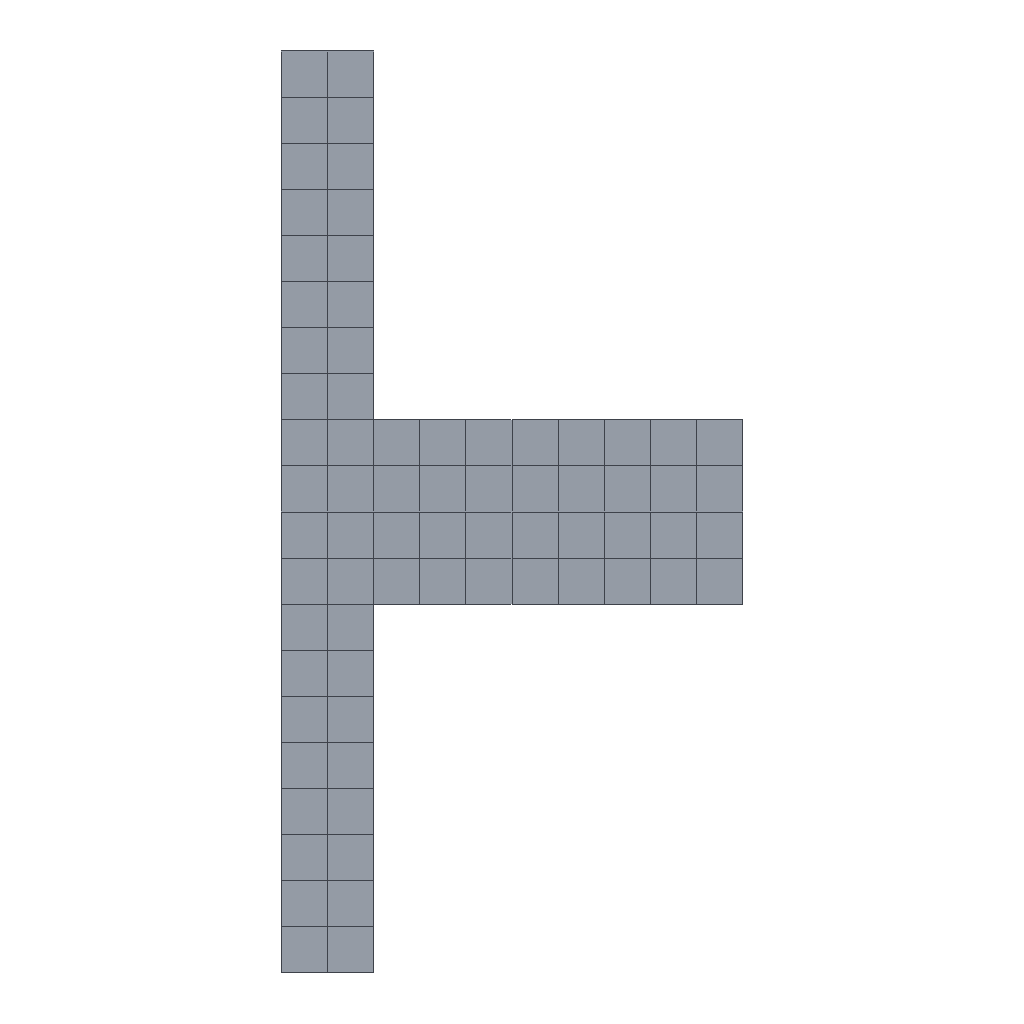Simulation study | abaqus
Set-up summary:
category,name,step,type,value,unit,region
solver,abaqus
solver,version,,,Abaqus/Standard 3DEXPERIENCE R2017x HotFix 2
units,not stated in the deck,,not stated
analysis,deck,,static,static
load_step,deadLoad,deadLoad,static
load_step,heat1,heat1,static
load_step,cool1,cool1,static
load_step,heat2,heat2,static
load_step,cool2,cool2,static
load_step,heat3,heat3,static
load_step,cool3,cool3,static
load_step,heat4,heat4,static
load_step,cool4,cool4,static
load_step,requested,,,9
mesh,nodes,,,114
mesh,elements,,,72
element_type,CAX4I,,axisymmetric,72
load,load commands in deck,,count,10
bc,support commands in deck,,count,2
material,STEEL,,in results
check,setup vs results,,match,"per instance, exact: element labels, types and connectivity; labels of the nodes the elements use; coordinates of those nodes at SINGLE_PRECISION in 2 of 2 instance(s)"
Abaqus input file, long lists of numbers shortened:
*Heading
 axisymmetric flange connection
** Job name: flange_iso Model name: flange_iso
** Generated by: Abaqus/CAE 2017.HF2
*Preprint, echo=NO, model=NO, history=NO, contact=NO
**
** PARTS
**
*Part, name=botFlange
*End Part
**
*Part, name=topFlange
*End Part
**
**
** ASSEMBLY
**
*Assembly, name=Assembly
**
*Instance, name=botFlange-1, part=botFlange
*Node
      1, 0.09, -0.02
      2,  0.13, -0.02
** (55 more lines like these left out)
*Element, type=CAX4I
1,  1, 10, 42,  4
2, 10, 11, 43, 42
** (34 more lines like these left out)
*Nset, nset=_PickedSet2, internal, generate
  1,  57,   1
*Elset, elset=_PickedSet2, internal, generate
  1,  36,   1
** Section: Section-1
*Solid Section, elset=_PickedSet2, material=steel
1.,
*End Instance
**
*Instance, name=topFlange-1, part=topFlange
*Node
      1, 0.09,           0.
      2,  0.13,           0.
** (55 more lines like these left out)
*Element, type=CAX4I
1,  1, 10, 42,  4
2, 10, 11, 43, 42
** (34 more lines like these left out)
*Nset, nset=_PickedSet2, internal, generate
  1,  57,   1
*Elset, elset=_PickedSet2, internal, generate
  1,  36,   1
** Section: Section-1
*Solid Section, elset=_PickedSet2, material=steel
1.,
*End Instance
**
*Nset, nset=all, instance=botFlange-1, generate
  1,  57,   1
*Nset, nset=all, instance=topFlange-1, generate
  1,  57,   1
*Elset, elset=all, instance=botFlange-1, generate
  1,  36,   1
*Elset, elset=all, instance=topFlange-1, generate
  1,  36,   1
*Nset, nset=botBolt, instance=botFlange-1
 4,
*Nset, nset=fix, instance=topFlange-1
 6,
*Nset, nset=topBolt, instance=topFlange-1
 4,
*Nset, nset=tops, instance=botFlange-1
  7,  8, 31
*Nset, nset=tops, instance=topFlange-1
  7,  8, 27
*Elset, elset=tops, instance=botFlange-1
 23, 24
*Elset, elset=tops, instance=topFlange-1
 26, 36
*Elset, elset=_botFlange_S3, internal, instance=botFlange-1
  5,  6,  7,  8, 31, 32, 33, 34, 35, 36
*Surface, type=ELEMENT, name=botFlange
_botFlange_S3, S3
*Elset, elset=_press_S3, internal, instance=botFlange-1
 23, 24
*Elset, elset=_press_S2, internal, instance=topFlange-1
 26, 36
*Surface, type=ELEMENT, name=press
_press_S3, S3
_press_S2, S2
*Elset, elset=_topFlange_S1, internal, instance=topFlange-1, generate
 1,  4,  1
*Elset, elset=_topFlange_S2, internal, instance=topFlange-1, generate
 10,  16,   2
*Elset, elset=_topFlange_S4, internal, instance=topFlange-1
 17, 27
*Surface, type=ELEMENT, name=topFlange
_topFlange_S1, S1
_topFlange_S2, S2
_topFlange_S4, S4
** Constraint: tie bolt 1
*Equation
2
topBolt, 1, 1.
botBolt, 1, -1.
** Constraint: tie bolt 2
*Equation
2
topBolt, 2, 1.
botBolt, 2, -1.
*End Assembly
**
** MATERIALS
**
*Material, name=steel
*Elastic
 2.10439e+11, 0.3
*Expansion
 2e-05,
*Plastic
 1.99917e+08,          0.
 2.10439e+08, 0.0003387
 2.15977e+08, 0.00054
 2.21515e+08, 0.000755
 2.27053e+08, 0.0009824
 2.32591e+08,  0.001221
 2.38128e+08,  0.001468
 2.43666e+08,  0.001724
 2.49204e+08,  0.001986
 2.54742e+08,  0.002254
  2.6028e+08,  0.002524
 2.65818e+08,  0.002797
 2.71356e+08,  0.003072
 2.76894e+08,  0.003348
 2.82431e+08,  0.003628
 2.87969e+08,  0.003911
 2.93507e+08,  0.004198
 2.99045e+08,  0.004491
 3.04583e+08,  0.00479
 3.10121e+08,  0.005095
 3.15659e+08,  0.005409
 3.21196e+08,  0.005731
 3.26734e+08,  0.006062
 3.32272e+08,  0.006402
  3.3781e+08,   0.006753
 3.43348e+08,  0.007115
 3.48886e+08,  0.007488
 3.54424e+08,  0.007873
 3.59962e+08,     0.00827
 3.65499e+08,  0.00868
 3.71037e+08,  0.009104
 3.76575e+08,   0.009541
 3.82113e+08,  0.009993
 3.87651e+08,   0.01046
 3.93189e+08,    0.01095
 3.98727e+08,   0.01145
 4.04265e+08,   0.01197
 4.09802e+08,   0.01252
  4.1534e+08,   0.01309
 4.20878e+08,   0.01368
** (24 more lines like these left out)
**
** INTERACTION PROPERTIES
**
*Surface Interaction, name=fric
1.,
*Friction, slip tolerance=0.005
 0.1,
*Surface Behavior, pressure-overclosure=HARD
**
** INTERACTIONS
**
** Interaction: Int-1
*Contact Pair, interaction=fric, small sliding
topFlange, botFlange
** ----------------------------------------------------------------
**
** STEP: deadLoad
**
*Step, name=deadLoad, nlgeom=YES
apply dead load of pipe weight
*Static
0.1, 1., 1e-05, 1.
**
** BOUNDARY CONDITIONS
**
** Name: fixRB Type: Displacement/Rotation
*Boundary
fix, 2, 2
**
** LOADS
**
** Name: Load-1   Type: Pressure
*Dsload
press, P, -4.9735e+07
**
** PREDEFINED FIELDS
**
** Name: Field-1   Type: Temperature
*Temperature
all, 20.
**
** OUTPUT REQUESTS
**
*Restart, write, frequency=0
**
** FIELD OUTPUT: F-Output-1
**
*Output, field, variable=PRESELECT
**
** HISTORY OUTPUT: H-Output-1
**
*Output, history, variable=PRESELECT
*End Step
** ----------------------------------------------------------------
**
** STEP: heat1
**
*Step, name=heat1, nlgeom=YES
1st heat up cycle
*Static
0.05, 1., 1e-05, 1.
**
** BOUNDARY CONDITIONS
**
** Name: fixRB Type: Displacement/Rotation
*Boundary, op=NEW
** Name: fixTops Type: Velocity/Angular velocity
*Boundary, op=NEW, type=VELOCITY
tops, 2, 2
**
** LOADS
**
** Name: Load-1   Type: Pressure
*Dsload, op=NEW
**
** PREDEFINED FIELDS
**
** Name: Field-1   Type: Temperature
*Temperature
all, 350.
**
** OUTPUT REQUESTS
**
*Restart, write, frequency=0
**
** FIELD OUTPUT: F-Output-1
**
*Output, field, variable=PRESELECT
**
** HISTORY OUTPUT: H-Output-1
**
*Output, history, variable=PRESELECT
*End Step
** ----------------------------------------------------------------
**
** STEP: cool1
**
*Step, name=cool1, nlgeom=YES
1st cooling cycle
*Static
0.05, 1., 1e-05, 1.
**
** PREDEFINED FIELDS
**
** Name: Field-1   Type: Temperature
*Temperature
all, 25.
**
** OUTPUT REQUESTS
**
*Restart, write, frequency=0
**
** FIELD OUTPUT: F-Output-1
**
*Output, field, variable=PRESELECT
**
** HISTORY OUTPUT: H-Output-1
**
*Output, history, variable=PRESELECT
*End Step
** ----------------------------------------------------------------
**
** STEP: heat2
**
*Step, name=heat2, nlgeom=YES
2nd heat up cycle
*Static
0.05, 1., 1e-05, 1.
**
** PREDEFINED FIELDS
**
** Name: Field-1   Type: Temperature
*Temperature
all, 350.
**
** OUTPUT REQUESTS
**
*Restart, write, frequency=0
**
** FIELD OUTPUT: F-Output-1
**
*Output, field, variable=PRESELECT
**
** HISTORY OUTPUT: H-Output-1
**
*Output, history, variable=PRESELECT
*End Step
** ----------------------------------------------------------------
**
** STEP: cool2
**
*Step, name=cool2, nlgeom=YES
2nd cooling cycle
*Static
0.05, 1., 1e-05, 1.
**
** PREDEFINED FIELDS
**
** Name: Field-1   Type: Temperature
*Temperature
all, 25.
**
** OUTPUT REQUESTS
**
*Restart, write, frequency=0
**
** FIELD OUTPUT: F-Output-1
**
*Output, field, variable=PRESELECT
**
** HISTORY OUTPUT: H-Output-1
**
*Output, history, variable=PRESELECT
*End Step
** ----------------------------------------------------------------
**
** STEP: heat3
**
*Step, name=heat3, nlgeom=YES
3rd heat up cycle
*Static
0.05, 1., 1e-05, 1.
**
** PREDEFINED FIELDS
**
** Name: Field-1   Type: Temperature
*Temperature
all, 350.
**
** OUTPUT REQUESTS
**
*Restart, write, frequency=0
**
** FIELD OUTPUT: F-Output-1
**
*Output, field, variable=PRESELECT
**
** HISTORY OUTPUT: H-Output-1
**
*Output, history, variable=PRESELECT
*End Step
** ----------------------------------------------------------------
**
** STEP: cool3
**
*Step, name=cool3, nlgeom=YES
3rd cooling cycle
*Static
0.05, 1., 1e-05, 1.
**
** PREDEFINED FIELDS
**
** Name: Field-1   Type: Temperature
*Temperature
all, 25.
**
** OUTPUT REQUESTS
**
*Restart, write, frequency=0
**
** FIELD OUTPUT: F-Output-1
**
*Output, field, variable=PRESELECT
**
** HISTORY OUTPUT: H-Output-1
**
*Output, history, variable=PRESELECT
*End Step
** ----------------------------------------------------------------
**
** STEP: heat4
**
*Step, name=heat4, nlgeom=YES
4th heat up cycle
*Static
0.05, 1., 1e-05, 1.
**
** PREDEFINED FIELDS
**
** Name: Field-1   Type: Temperature
*Temperature
all, 350.
**
** OUTPUT REQUESTS
**
*Restart, write, frequency=0
**
** FIELD OUTPUT: F-Output-1
**
*Output, field, variable=PRESELECT
**
** HISTORY OUTPUT: H-Output-1
**
*Output, history, variable=PRESELECT
*End Step
** ----------------------------------------------------------------
**
** STEP: cool4
**
*Step, name=cool4, nlgeom=YES
4th cooling cycle
*Static
0.05, 1., 1e-05, 1.
**
** PREDEFINED FIELDS
**
** Name: Field-1   Type: Temperature
*Temperature
all, 25.
**
** OUTPUT REQUESTS
**
*Restart, write, frequency=0
**
** FIELD OUTPUT: F-Output-1
**
*Output, field, variable=PRESELECT
**
** HISTORY OUTPUT: H-Output-1
**
*Output, history, variable=PRESELECT
*End Step
Results summary:
result,step,apply dead load of pipe weight,completed,increments=6 time=1.0/1.0
result,step,1st heat up cycle,completed,increments=7 time=1.0/1.0
result,step,1st cooling cycle,completed,increments=7 time=1.0/1.0
result,step,2nd heat up cycle,completed,increments=7 time=1.0/1.0
result,step,2nd cooling cycle,completed,increments=7 time=1.0/1.0
result,step,3rd heat up cycle,completed,increments=7 time=1.0/1.0
result,step,3rd cooling cycle,completed,increments=7 time=1.0/1.0
result,step,4th heat up cycle,completed,increments=7 time=1.0/1.0
result,step,4th cooling cycle,completed,increments=7 time=1.0/1.0
result,analysis,,,static
result,last_loadstep,,,9
result,primary field,,,U
result,reaction total,,FX,0.0,model units
result,reaction total,,FY,0.0,model units
result,reaction total,,FZ,0.0,model units